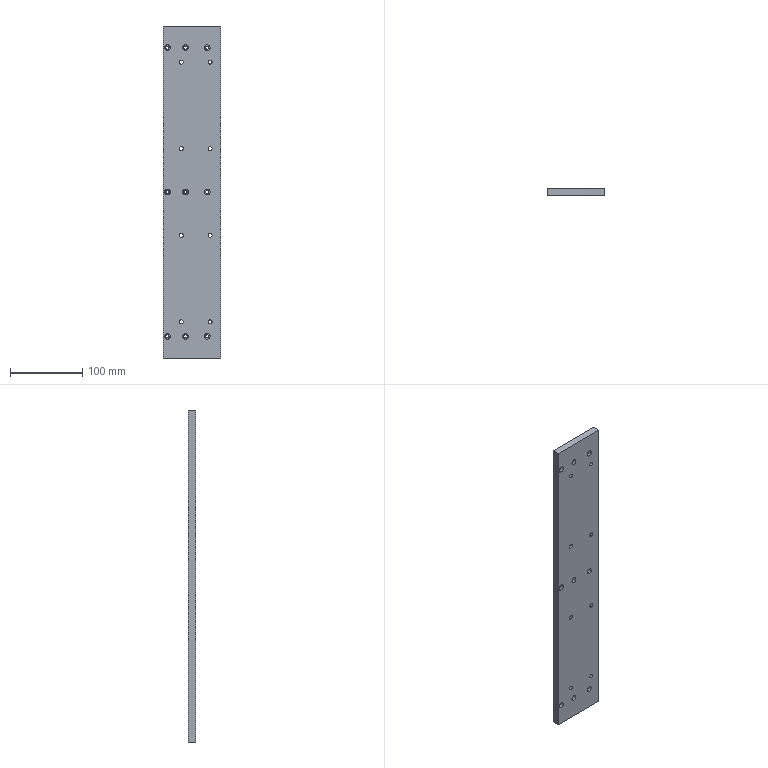Part | SolidWorks | features HoleWzd 2, Extrusion 1 | 1 solid | 91 faces | box 80 x 10 x 460 mm | volume 360747 mm3 | cylinder 68 | plane 23 | commonest cylinder face diameters 4.5 x18 8 x18 5.5 x16 10 x16